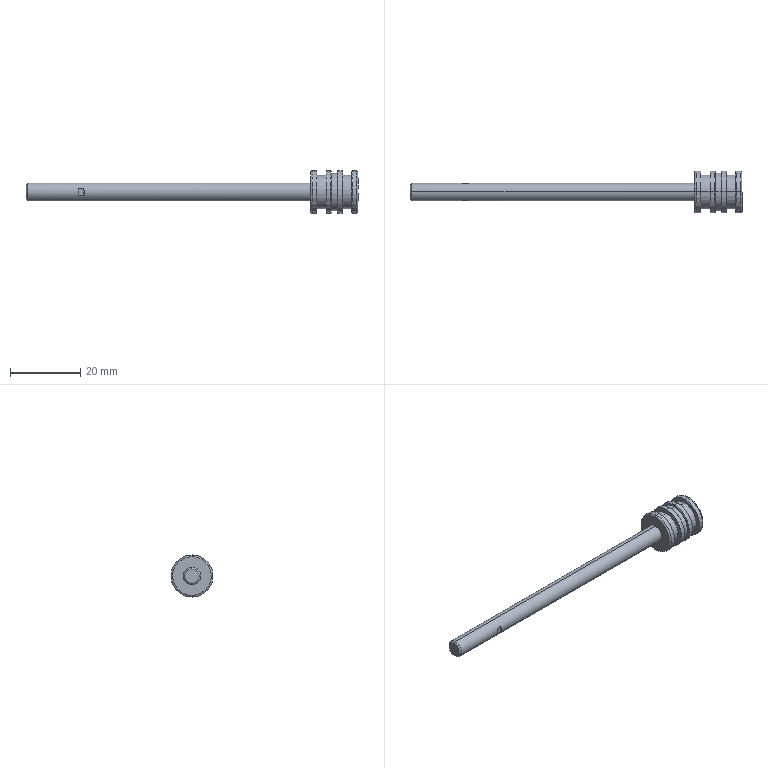Part | STEP file | PBR12X30SU-02-CC | 1 solid | 49 faces | box 94.5 x 12 x 12 mm | volume 2851 mm3 | cylinder 16 | plane 15 | cone 14 | spline 4 | commonest cylinder face diameters 12 x8 9.5 x4 5 x2 10.7 x2